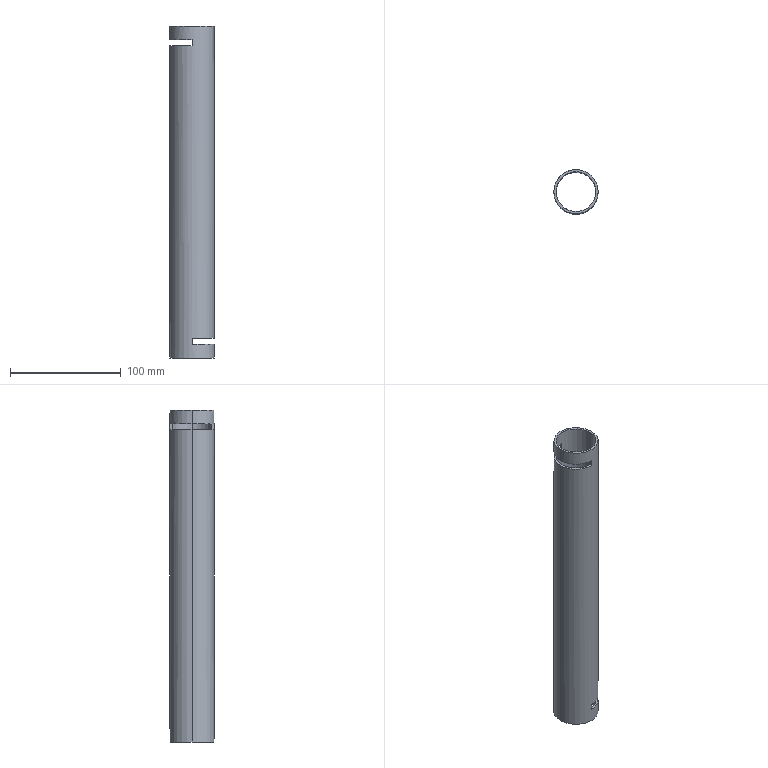Part | STEP file | Support tube | 1 solid | 14 faces | box 40 x 40 x 300 mm | volume 70315 mm3 | plane 10 | cylinder 4 | commonest cylinder face diameters 36 x2 40 x2